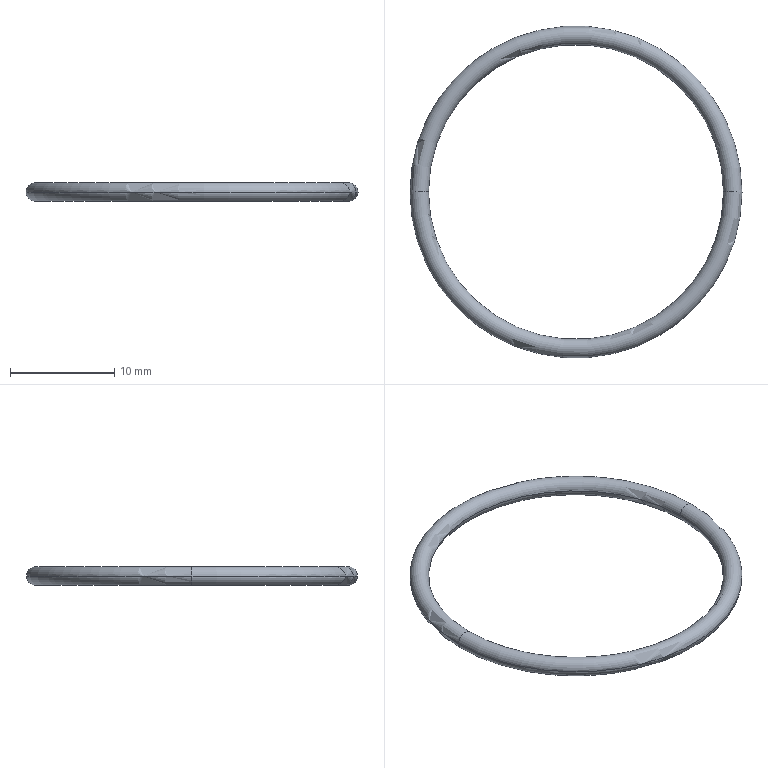Part | NX | features REVOLVE1 2 | 1 solid | 4 faces | box 31.852 x 31.852 x 1.778 mm | volume 234.579 mm3 | torus 4
STEP:
#1=CARTESIAN_POINT('',(-15.926,0.,0.));
#2=VERTEX_POINT('',#1);
#3=CARTESIAN_POINT('',(-14.148,0.,0.));
#4=VERTEX_POINT('',#3);
#5=CARTESIAN_POINT('',(-15.037,0.,0.));
#6=DIRECTION('',(0.,1.,0.));
#7=DIRECTION('',(-1.,0.,0.));
#8=AXIS2_PLACEMENT_3D('',#5,#6,#7);
#9=CIRCLE('',#8,0.889);
#10=EDGE_CURVE('',#2,#4,#9,.T.);
#11=ORIENTED_EDGE('',*,*,#10,.F.);
#12=CARTESIAN_POINT('',(15.926,0.,0.));
#13=VERTEX_POINT('',#12);
#14=CARTESIAN_POINT('',(0.,0.,0.));
#15=DIRECTION('',(0.,0.,1.));
#16=DIRECTION('',(1.,0.,0.));
#17=AXIS2_PLACEMENT_3D('',#14,#15,#16);
#18=CIRCLE('',#17,15.926);
#19=EDGE_CURVE('',#2,#13,#18,.T.);
#20=ORIENTED_EDGE('',*,*,#19,.T.);
#21=CARTESIAN_POINT('',(14.148,0.,0.));
#22=VERTEX_POINT('',#21);
#23=CARTESIAN_POINT('',(15.037,0.,0.));
#24=DIRECTION('',(0.,-1.,0.));
#25=DIRECTION('',(0.,0.,-1.));
#26=AXIS2_PLACEMENT_3D('',#23,#24,#25);
#27=CIRCLE('',#26,0.889);
#28=EDGE_CURVE('',#22,#13,#27,.F.);
#29=ORIENTED_EDGE('',*,*,#28,.F.);
#30=CARTESIAN_POINT('',(0.,0.,0.));
#31=DIRECTION('',(0.,0.,1.));
#32=DIRECTION('',(1.,0.,0.));
#33=AXIS2_PLACEMENT_3D('',#30,#31,#32);
#34=CIRCLE('',#33,14.148);
#35=EDGE_CURVE('',#22,#4,#34,.F.);
#36=ORIENTED_EDGE('',*,*,#35,.T.);
#37=EDGE_LOOP('',(#11,#20,#29,#36));
#38=FACE_BOUND('',#37,.T.);
#39=CARTESIAN_POINT('',(0.,0.,0.));
#40=DIRECTION('',(0.,0.,1.));
#41=DIRECTION('',(-1.,0.,0.));
#42=AXIS2_PLACEMENT_3D('',#39,#40,#41);
#43=TOROIDAL_SURFACE('',#42,15.037,0.889);
#44=ADVANCED_FACE('',(#38),#43,.T.);
#45=ORIENTED_EDGE('',*,*,#28,.T.);
#46=CARTESIAN_POINT('',(0.,0.,0.));
#47=DIRECTION('',(0.,0.,1.));
#48=DIRECTION('',(1.,0.,0.));
#49=AXIS2_PLACEMENT_3D('',#46,#47,#48);
#50=CIRCLE('',#49,15.926);
#51=EDGE_CURVE('',#13,#2,#50,.T.);
#52=ORIENTED_EDGE('',*,*,#51,.T.);
#53=ORIENTED_EDGE('',*,*,#10,.T.);
#54=CARTESIAN_POINT('',(0.,0.,0.));
#55=DIRECTION('',(0.,0.,1.));
#56=DIRECTION('',(1.,0.,0.));
#57=AXIS2_PLACEMENT_3D('',#54,#55,#56);
#58=CIRCLE('',#57,14.148);
#59=EDGE_CURVE('',#4,#22,#58,.F.);
#60=ORIENTED_EDGE('',*,*,#59,.T.);
#61=EDGE_LOOP('',(#45,#52,#53,#60));
#62=FACE_BOUND('',#61,.T.);
#63=CARTESIAN_POINT('',(0.,0.,0.));
#64=DIRECTION('',(0.,0.,1.));
#65=DIRECTION('',(-1.,0.,0.));
#66=AXIS2_PLACEMENT_3D('',#63,#64,#65);
#67=TOROIDAL_SURFACE('',#66,15.037,0.889);
#68=ADVANCED_FACE('',(#62),#67,.T.);
#69=ORIENTED_EDGE('',*,*,#51,.F.);
#70=CARTESIAN_POINT('',(15.037,0.,0.));
#71=DIRECTION('',(0.,-1.,0.));
#72=DIRECTION('',(0.,0.,-1.));
#73=AXIS2_PLACEMENT_3D('',#70,#71,#72);
#74=CIRCLE('',#73,0.889);
#75=EDGE_CURVE('',#22,#13,#74,.T.);
#76=ORIENTED_EDGE('',*,*,#75,.F.);
#77=ORIENTED_EDGE('',*,*,#59,.F.);
#78=CARTESIAN_POINT('',(-15.037,0.,0.));
#79=DIRECTION('',(0.,1.,0.));
#80=DIRECTION('',(-1.,0.,0.));
#81=AXIS2_PLACEMENT_3D('',#78,#79,#80);
#82=CIRCLE('',#81,0.889);
#83=EDGE_CURVE('',#2,#4,#82,.F.);
#84=ORIENTED_EDGE('',*,*,#83,.F.);
#85=EDGE_LOOP('',(#69,#76,#77,#84));
#86=FACE_BOUND('',#85,.T.);
#87=CARTESIAN_POINT('',(0.,0.,0.));
#88=DIRECTION('',(0.,0.,1.));
#89=DIRECTION('',(-1.,0.,0.));
#90=AXIS2_PLACEMENT_3D('',#87,#88,#89);
#91=TOROIDAL_SURFACE('',#90,15.037,0.889);
#92=ADVANCED_FACE('',(#86),#91,.T.);
#93=ORIENTED_EDGE('',*,*,#19,.F.);
#94=ORIENTED_EDGE('',*,*,#83,.T.);
#95=ORIENTED_EDGE('',*,*,#35,.F.);
#96=ORIENTED_EDGE('',*,*,#75,.T.);
#97=EDGE_LOOP('',(#93,#94,#95,#96));
#98=FACE_BOUND('',#97,.T.);
#99=CARTESIAN_POINT('',(0.,0.,0.));
#100=DIRECTION('',(0.,0.,1.));
#101=DIRECTION('',(-1.,0.,0.));
#102=AXIS2_PLACEMENT_3D('',#99,#100,#101);
#103=TOROIDAL_SURFACE('',#102,15.037,0.889);
#104=ADVANCED_FACE('',(#98),#103,.T.);
#105=CLOSED_SHELL('',(#44,#68,#92,#104));
#106=MANIFOLD_SOLID_BREP('',#105);
#107=(LENGTH_UNIT()NAMED_UNIT(*)SI_UNIT(.MILLI.,.METRE.));
#108=UNCERTAINTY_MEASURE_WITH_UNIT(LENGTH_MEASURE(0.00001),#107,'','');
#109=(NAMED_UNIT(*)PLANE_ANGLE_UNIT()SI_UNIT($,.RADIAN.));
#110=(NAMED_UNIT(*)SI_UNIT($,.STERADIAN.)SOLID_ANGLE_UNIT());
#111=(GEOMETRIC_REPRESENTATION_CONTEXT(3)GLOBAL_UNCERTAINTY_ASSIGNED_CONTEXT((#108))GLOBAL_UNIT_ASSIGNED_CONTEXT((#107,#109,#110))REPRESENTATION_CONTEXT('',''));
#112=ADVANCED_BREP_SHAPE_REPRESENTATION('',(#106),#111);